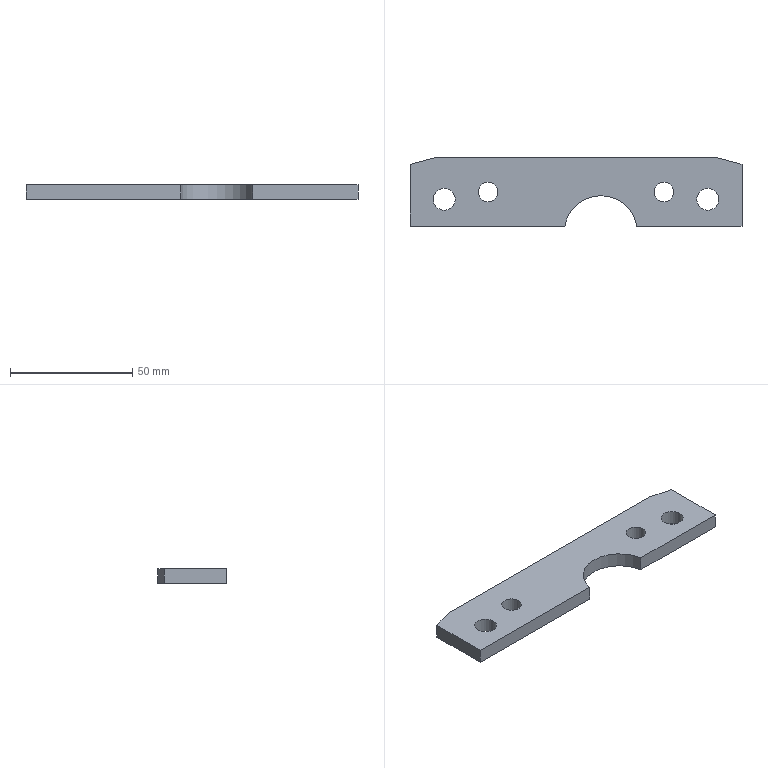Part | STEP file | gslz 2016.10.28-13_id714_x_t | 1 solid | 14 faces | box 136 x 28 x 6 mm | volume 19648 mm3 | plane 9 | cylinder 5 | commonest cylinder face diameters 8 x2 9 x2 30 x1
STEP:
#1=CARTESIAN_POINT('',(0.,0.,0.));
#2=DIRECTION('',(0.,0.,1.));
#3=DIRECTION('',(1.,0.,0.));
#4=AXIS2_PLACEMENT_3D('',#1,#2,#3);
#5=CARTESIAN_POINT('',(-122.555,-295.75,6.));
#6=VERTEX_POINT('',#5);
#7=CARTESIAN_POINT('',(-79.516,-295.75,6.));
#8=VERTEX_POINT('',#7);
#9=CARTESIAN_POINT('',(-142.516,-295.75,6.));
#10=DIRECTION('',(1.,0.,0.));
#11=VECTOR('',#10,1.);
#12=LINE('',#9,#11);
#13=CARTESIAN_POINT('',(-142.516,-295.75,16.));
#14=DIRECTION('',(0.,1.,0.));
#15=DIRECTION('',(0.,0.,-1.));
#16=AXIS2_PLACEMENT_3D('',#13,#14,#15);
#17=PLANE('',#16);
#18=CARTESIAN_POINT('',(10.,0.));
#19=DIRECTION('',(0.,-1.));
#20=VECTOR('',#19,1.);
#21=LINE('',#18,#20);
#22=(GEOMETRIC_REPRESENTATION_CONTEXT(2)PARAMETRIC_REPRESENTATION_CONTEXT()REPRESENTATION_CONTEXT('',''));
#23=DEFINITIONAL_REPRESENTATION('',(#21),#22);
#24=PCURVE('',#17,#23);
#25=CARTESIAN_POINT('',(-182.516,-265.25,6.));
#26=DIRECTION('',(0.,0.,-1.));
#27=DIRECTION('',(-1.,0.,0.));
#28=AXIS2_PLACEMENT_3D('',#25,#26,#27);
#29=PLANE('',#28);
#30=CARTESIAN_POINT('',(-40.,-30.5));
#31=DIRECTION('',(-1.,0.));
#32=VECTOR('',#31,1.);
#33=LINE('',#30,#32);
#34=(GEOMETRIC_REPRESENTATION_CONTEXT(2)PARAMETRIC_REPRESENTATION_CONTEXT()REPRESENTATION_CONTEXT('',''));
#35=DEFINITIONAL_REPRESENTATION('',(#33),#34);
#36=PCURVE('',#29,#35);
#37=SURFACE_CURVE('',#12,(#24,#36),.PCURVE_S1.);
#38=EDGE_CURVE('',#6,#8,#37,.T.);
#39=ORIENTED_EDGE('',*,*,#38,.F.);
#40=CARTESIAN_POINT('',(-122.555,-295.75,0.));
#41=VERTEX_POINT('',#40);
#42=CARTESIAN_POINT('',(-122.555,-295.75,290.));
#43=DIRECTION('',(0.,0.,-1.));
#44=VECTOR('',#43,1.);
#45=LINE('',#42,#44);
#46=CARTESIAN_POINT('',(-274.,-19.961));
#47=DIRECTION('',(1.,0.));
#48=VECTOR('',#47,1.);
#49=LINE('',#46,#48);
#50=(GEOMETRIC_REPRESENTATION_CONTEXT(2)PARAMETRIC_REPRESENTATION_CONTEXT()REPRESENTATION_CONTEXT('',''));
#51=DEFINITIONAL_REPRESENTATION('',(#49),#50);
#52=PCURVE('',#17,#51);
#53=CARTESIAN_POINT('',(-137.345,-298.25,290.));
#54=DIRECTION('',(0.,0.,-1.));
#55=DIRECTION('',(-1.,0.,0.));
#56=AXIS2_PLACEMENT_3D('',#53,#54,#55);
#57=CYLINDRICAL_SURFACE('',#56,15.);
#58=CARTESIAN_POINT('',(2.974,0.));
#59=DIRECTION('',(0.,1.));
#60=VECTOR('',#59,1.);
#61=LINE('',#58,#60);
#62=(GEOMETRIC_REPRESENTATION_CONTEXT(2)PARAMETRIC_REPRESENTATION_CONTEXT()REPRESENTATION_CONTEXT('',''));
#63=DEFINITIONAL_REPRESENTATION('',(#61),#62);
#64=PCURVE('',#57,#63);
#65=SURFACE_CURVE('',#45,(#52,#64),.PCURVE_S1.);
#66=EDGE_CURVE('',#6,#41,#65,.T.);
#67=ORIENTED_EDGE('',*,*,#66,.T.);
#68=CARTESIAN_POINT('',(-79.516,-295.75,0.));
#69=VERTEX_POINT('',#68);
#70=CARTESIAN_POINT('',(-142.516,-295.75,0.));
#71=DIRECTION('',(-1.,0.,0.));
#72=VECTOR('',#71,1.);
#73=LINE('',#70,#72);
#74=CARTESIAN_POINT('',(16.,0.));
#75=DIRECTION('',(0.,1.));
#76=VECTOR('',#75,1.);
#77=LINE('',#74,#76);
#78=(GEOMETRIC_REPRESENTATION_CONTEXT(2)PARAMETRIC_REPRESENTATION_CONTEXT()REPRESENTATION_CONTEXT('',''));
#79=DEFINITIONAL_REPRESENTATION('',(#77),#78);
#80=PCURVE('',#17,#79);
#81=CARTESIAN_POINT('',(-222.516,-295.75,0.));
#82=DIRECTION('',(0.,0.,1.));
#83=DIRECTION('',(1.,0.,0.));
#84=AXIS2_PLACEMENT_3D('',#81,#82,#83);
#85=PLANE('',#84);
#86=CARTESIAN_POINT('',(80.,0.));
#87=DIRECTION('',(-1.,0.));
#88=VECTOR('',#87,1.);
#89=LINE('',#86,#88);
#90=(GEOMETRIC_REPRESENTATION_CONTEXT(2)PARAMETRIC_REPRESENTATION_CONTEXT()REPRESENTATION_CONTEXT('',''));
#91=DEFINITIONAL_REPRESENTATION('',(#89),#90);
#92=PCURVE('',#85,#91);
#93=SURFACE_CURVE('',#73,(#80,#92),.PCURVE_S1.);
#94=EDGE_CURVE('',#69,#41,#93,.T.);
#95=ORIENTED_EDGE('',*,*,#94,.F.);
#96=CARTESIAN_POINT('',(-79.516,-295.75,16.));
#97=DIRECTION('',(0.,0.,-1.));
#98=VECTOR('',#97,1.);
#99=LINE('',#96,#98);
#100=CARTESIAN_POINT('',(0.,-63.));
#101=DIRECTION('',(1.,0.));
#102=VECTOR('',#101,1.);
#103=LINE('',#100,#102);
#104=(GEOMETRIC_REPRESENTATION_CONTEXT(2)PARAMETRIC_REPRESENTATION_CONTEXT()REPRESENTATION_CONTEXT('',''));
#105=DEFINITIONAL_REPRESENTATION('',(#103),#104);
#106=PCURVE('',#17,#105);
#107=CARTESIAN_POINT('',(-79.516,-262.75,16.));
#108=DIRECTION('',(-1.,0.,0.));
#109=DIRECTION('',(0.,0.,1.));
#110=AXIS2_PLACEMENT_3D('',#107,#108,#109);
#111=PLANE('',#110);
#112=CARTESIAN_POINT('',(0.,-33.));
#113=DIRECTION('',(-1.,0.));
#114=VECTOR('',#113,1.);
#115=LINE('',#112,#114);
#116=(GEOMETRIC_REPRESENTATION_CONTEXT(2)PARAMETRIC_REPRESENTATION_CONTEXT()REPRESENTATION_CONTEXT('',''));
#117=DEFINITIONAL_REPRESENTATION('',(#115),#116);
#118=PCURVE('',#111,#117);
#119=SURFACE_CURVE('',#99,(#106,#118),.PCURVE_S1.);
#120=EDGE_CURVE('',#8,#69,#119,.T.);
#121=ORIENTED_EDGE('',*,*,#120,.F.);
#122=EDGE_LOOP('',(#39,#67,#95,#121));
#123=FACE_BOUND('',#122,.T.);
#124=ADVANCED_FACE('',(#123),#17,.F.);
#125=CARTESIAN_POINT('',(-89.016,-284.75,0.));
#126=VERTEX_POINT('',#125);
#127=CARTESIAN_POINT('',(-98.016,-284.75,0.));
#128=VERTEX_POINT('',#127);
#129=CARTESIAN_POINT('',(-93.516,-284.75,0.));
#130=DIRECTION('',(0.,0.,1.));
#131=DIRECTION('',(1.,0.,0.));
#132=AXIS2_PLACEMENT_3D('',#129,#130,#131);
#133=CIRCLE('',#132,4.5);
#134=CARTESIAN_POINT('',(129.,11.));
#135=DIRECTION('',(1.,0.));
#136=AXIS2_PLACEMENT_2D('',#134,#135);
#137=CIRCLE('',#136,4.5);
#138=(GEOMETRIC_REPRESENTATION_CONTEXT(2)PARAMETRIC_REPRESENTATION_CONTEXT()REPRESENTATION_CONTEXT('',''));
#139=DEFINITIONAL_REPRESENTATION('',(#137),#138);
#140=PCURVE('',#85,#139);
#141=CARTESIAN_POINT('',(-93.516,-284.75,47.));
#142=DIRECTION('',(0.,0.,-1.));
#143=DIRECTION('',(-1.,0.,0.));
#144=AXIS2_PLACEMENT_3D('',#141,#142,#143);
#145=CYLINDRICAL_SURFACE('',#144,4.5);
#146=CARTESIAN_POINT('',(3.142,47.));
#147=DIRECTION('',(-1.,0.));
#148=VECTOR('',#147,1.);
#149=LINE('',#146,#148);
#150=(GEOMETRIC_REPRESENTATION_CONTEXT(2)PARAMETRIC_REPRESENTATION_CONTEXT()REPRESENTATION_CONTEXT('',''));
#151=DEFINITIONAL_REPRESENTATION('',(#149),#150);
#152=PCURVE('',#145,#151);
#153=SURFACE_CURVE('',#133,(#140,#152),.PCURVE_S1.);
#154=EDGE_CURVE('',#126,#128,#153,.T.);
#155=ORIENTED_EDGE('',*,*,#154,.T.);
#156=CARTESIAN_POINT('',(-93.516,-284.75,0.));
#157=DIRECTION('',(0.,0.,1.));
#158=DIRECTION('',(1.,0.,0.));
#159=AXIS2_PLACEMENT_3D('',#156,#157,#158);
#160=CIRCLE('',#159,4.5);
#161=CARTESIAN_POINT('',(129.,11.));
#162=DIRECTION('',(1.,0.));
#163=AXIS2_PLACEMENT_2D('',#161,#162);
#164=CIRCLE('',#163,4.5);
#165=(GEOMETRIC_REPRESENTATION_CONTEXT(2)PARAMETRIC_REPRESENTATION_CONTEXT()REPRESENTATION_CONTEXT('',''));
#166=DEFINITIONAL_REPRESENTATION('',(#164),#165);
#167=PCURVE('',#85,#166);
#168=CARTESIAN_POINT('',(9.425,47.));
#169=DIRECTION('',(-1.,0.));
#170=VECTOR('',#169,1.);
#171=LINE('',#168,#170);
#172=(GEOMETRIC_REPRESENTATION_CONTEXT(2)PARAMETRIC_REPRESENTATION_CONTEXT()REPRESENTATION_CONTEXT('',''));
#173=DEFINITIONAL_REPRESENTATION('',(#171),#172);
#174=PCURVE('',#145,#173);
#175=SURFACE_CURVE('',#160,(#167,#174),.PCURVE_S1.);
#176=EDGE_CURVE('',#128,#126,#175,.T.);
#177=ORIENTED_EDGE('',*,*,#176,.T.);
#178=EDGE_LOOP('',(#155,#177));
#179=FACE_BOUND('',#178,.T.);
#180=CARTESIAN_POINT('',(-179.516,-281.75,0.));
#181=VERTEX_POINT('',#180);
#182=CARTESIAN_POINT('',(-183.516,-281.75,0.));
#183=DIRECTION('',(0.,0.,1.));
#184=DIRECTION('',(1.,0.,0.));
#185=AXIS2_PLACEMENT_3D('',#182,#183,#184);
#186=CIRCLE('',#185,4.);
#187=CARTESIAN_POINT('',(39.,14.));
#188=DIRECTION('',(1.,0.));
#189=AXIS2_PLACEMENT_2D('',#187,#188);
#190=CIRCLE('',#189,4.);
#191=(GEOMETRIC_REPRESENTATION_CONTEXT(2)PARAMETRIC_REPRESENTATION_CONTEXT()REPRESENTATION_CONTEXT('',''));
#192=DEFINITIONAL_REPRESENTATION('',(#190),#191);
#193=PCURVE('',#85,#192);
#194=CARTESIAN_POINT('',(-183.516,-281.75,-73.));
#195=DIRECTION('',(0.,0.,1.));
#196=DIRECTION('',(1.,0.,0.));
#197=AXIS2_PLACEMENT_3D('',#194,#195,#196);
#198=CYLINDRICAL_SURFACE('',#197,4.);
#199=CARTESIAN_POINT('',(0.,73.));
#200=DIRECTION('',(1.,0.));
#201=VECTOR('',#200,1.);
#202=LINE('',#199,#201);
#203=(GEOMETRIC_REPRESENTATION_CONTEXT(2)PARAMETRIC_REPRESENTATION_CONTEXT()REPRESENTATION_CONTEXT('',''));
#204=DEFINITIONAL_REPRESENTATION('',(#202),#203);
#205=PCURVE('',#198,#204);
#206=SURFACE_CURVE('',#186,(#193,#205),.PCURVE_S1.);
#207=EDGE_CURVE('',#181,#181,#206,.T.);
#208=ORIENTED_EDGE('',*,*,#207,.T.);
#209=EDGE_LOOP('',(#208));
#210=FACE_BOUND('',#209,.T.);
#211=CARTESIAN_POINT('',(-107.516,-281.75,0.));
#212=VERTEX_POINT('',#211);
#213=CARTESIAN_POINT('',(-111.516,-281.75,0.));
#214=DIRECTION('',(0.,0.,-1.));
#215=DIRECTION('',(1.,0.,0.));
#216=AXIS2_PLACEMENT_3D('',#213,#214,#215);
#217=CIRCLE('',#216,4.);
#218=CARTESIAN_POINT('',(115.,14.));
#219=CARTESIAN_POINT('',(115.,7.072));
#220=CARTESIAN_POINT('',(109.,10.536));
#221=CARTESIAN_POINT('',(103.,14.));
#222=CARTESIAN_POINT('',(109.,17.464));
#223=CARTESIAN_POINT('',(115.,20.928));
#224=CARTESIAN_POINT('',(115.,14.));
#225=(BOUNDED_CURVE()B_SPLINE_CURVE(2,(#218,#219,#220,#221,#222,#223,#224),.UNSPECIFIED.,.T.,.F.)B_SPLINE_CURVE_WITH_KNOTS((1,2,2,2,2,1),(-2.094,0.,2.094,4.189,6.283,8.378),.UNSPECIFIED.)CURVE()GEOMETRIC_REPRESENTATION_ITEM()RATIONAL_B_SPLINE_CURVE((1.,0.5,1.,0.5,1.,0.5,1.))REPRESENTATION_ITEM(''));
#226=(GEOMETRIC_REPRESENTATION_CONTEXT(2)PARAMETRIC_REPRESENTATION_CONTEXT()REPRESENTATION_CONTEXT('',''));
#227=DEFINITIONAL_REPRESENTATION('',(#225),#226);
#228=PCURVE('',#85,#227);
#229=CARTESIAN_POINT('',(-111.516,-281.75,-73.));
#230=DIRECTION('',(0.,0.,1.));
#231=DIRECTION('',(1.,0.,0.));
#232=AXIS2_PLACEMENT_3D('',#229,#230,#231);
#233=CYLINDRICAL_SURFACE('',#232,4.);
#234=CARTESIAN_POINT('',(6.283,73.));
#235=DIRECTION('',(-1.,0.));
#236=VECTOR('',#235,1.);
#237=LINE('',#234,#236);
#238=(GEOMETRIC_REPRESENTATION_CONTEXT(2)PARAMETRIC_REPRESENTATION_CONTEXT()REPRESENTATION_CONTEXT('',''));
#239=DEFINITIONAL_REPRESENTATION('',(#237),#238);
#240=PCURVE('',#233,#239);
#241=SURFACE_CURVE('',#217,(#228,#240),.PCURVE_S1.);
#242=EDGE_CURVE('',#212,#212,#241,.T.);
#243=ORIENTED_EDGE('',*,*,#242,.F.);
#244=EDGE_LOOP('',(#243));
#245=FACE_BOUND('',#244,.T.);
#246=CARTESIAN_POINT('',(-197.016,-284.75,0.));
#247=VERTEX_POINT('',#246);
#248=CARTESIAN_POINT('',(-206.016,-284.75,0.));
#249=VERTEX_POINT('',#248);
#250=CARTESIAN_POINT('',(-201.516,-284.75,0.));
#251=DIRECTION('',(0.,0.,-1.));
#252=DIRECTION('',(1.,0.,0.));
#253=AXIS2_PLACEMENT_3D('',#250,#251,#252);
#254=CIRCLE('',#253,4.5);
#255=CARTESIAN_POINT('',(25.5,11.));
#256=CARTESIAN_POINT('',(25.5,3.206));
#257=CARTESIAN_POINT('',(18.75,7.103));
#258=CARTESIAN_POINT('',(12.,11.));
#259=CARTESIAN_POINT('',(18.75,14.897));
#260=CARTESIAN_POINT('',(25.5,18.794));
#261=CARTESIAN_POINT('',(25.5,11.));
#262=(BOUNDED_CURVE()B_SPLINE_CURVE(2,(#255,#256,#257,#258,#259,#260,#261),.UNSPECIFIED.,.T.,.F.)B_SPLINE_CURVE_WITH_KNOTS((1,2,2,2,2,1),(-2.094,0.,2.094,4.189,6.283,8.378),.UNSPECIFIED.)CURVE()GEOMETRIC_REPRESENTATION_ITEM()RATIONAL_B_SPLINE_CURVE((1.,0.5,1.,0.5,1.,0.5,1.))REPRESENTATION_ITEM(''));
#263=(GEOMETRIC_REPRESENTATION_CONTEXT(2)PARAMETRIC_REPRESENTATION_CONTEXT()REPRESENTATION_CONTEXT('',''));
#264=DEFINITIONAL_REPRESENTATION('',(#262),#263);
#265=PCURVE('',#85,#264);
#266=CARTESIAN_POINT('',(-201.516,-284.75,47.));
#267=DIRECTION('',(0.,0.,-1.));
#268=DIRECTION('',(-1.,0.,0.));
#269=AXIS2_PLACEMENT_3D('',#266,#267,#268);
#270=CYLINDRICAL_SURFACE('',#269,4.5);
#271=CARTESIAN_POINT('',(3.142,47.));
#272=DIRECTION('',(1.,0.));
#273=VECTOR('',#272,1.);
#274=LINE('',#271,#273);
#275=(GEOMETRIC_REPRESENTATION_CONTEXT(2)PARAMETRIC_REPRESENTATION_CONTEXT()REPRESENTATION_CONTEXT('',''));
#276=DEFINITIONAL_REPRESENTATION('',(#274),#275);
#277=PCURVE('',#270,#276);
#278=SURFACE_CURVE('',#254,(#265,#277),.PCURVE_S1.);
#279=EDGE_CURVE('',#247,#249,#278,.T.);
#280=ORIENTED_EDGE('',*,*,#279,.F.);
#281=CARTESIAN_POINT('',(-201.516,-284.75,0.));
#282=DIRECTION('',(0.,0.,-1.));
#283=DIRECTION('',(1.,0.,0.));
#284=AXIS2_PLACEMENT_3D('',#281,#282,#283);
#285=CIRCLE('',#284,4.5);
#286=CARTESIAN_POINT('',(25.5,11.));
#287=CARTESIAN_POINT('',(25.5,3.206));
#288=CARTESIAN_POINT('',(18.75,7.103));
#289=CARTESIAN_POINT('',(12.,11.));
#290=CARTESIAN_POINT('',(18.75,14.897));
#291=CARTESIAN_POINT('',(25.5,18.794));
#292=CARTESIAN_POINT('',(25.5,11.));
#293=(BOUNDED_CURVE()B_SPLINE_CURVE(2,(#286,#287,#288,#289,#290,#291,#292),.UNSPECIFIED.,.T.,.F.)B_SPLINE_CURVE_WITH_KNOTS((1,2,2,2,2,1),(-2.094,0.,2.094,4.189,6.283,8.378),.UNSPECIFIED.)CURVE()GEOMETRIC_REPRESENTATION_ITEM()RATIONAL_B_SPLINE_CURVE((1.,0.5,1.,0.5,1.,0.5,1.))REPRESENTATION_ITEM(''));
#294=(GEOMETRIC_REPRESENTATION_CONTEXT(2)PARAMETRIC_REPRESENTATION_CONTEXT()REPRESENTATION_CONTEXT('',''));
#295=DEFINITIONAL_REPRESENTATION('',(#293),#294);
#296=PCURVE('',#85,#295);
#297=CARTESIAN_POINT('',(-3.142,47.));
#298=DIRECTION('',(1.,0.));
#299=VECTOR('',#298,1.);
#300=LINE('',#297,#299);
#301=(GEOMETRIC_REPRESENTATION_CONTEXT(2)PARAMETRIC_REPRESENTATION_CONTEXT()REPRESENTATION_CONTEXT('',''));
#302=DEFINITIONAL_REPRESENTATION('',(#300),#301);
#303=PCURVE('',#270,#302);
#304=SURFACE_CURVE('',#285,(#296,#303),.PCURVE_S1.);
#305=EDGE_CURVE('',#249,#247,#304,.T.);
#306=ORIENTED_EDGE('',*,*,#305,.F.);
#307=EDGE_LOOP('',(#280,#306));
#308=FACE_BOUND('',#307,.T.);
#309=CARTESIAN_POINT('',(-152.135,-295.75,0.));
#310=VERTEX_POINT('',#309);
#311=CARTESIAN_POINT('',(-137.345,-298.25,0.));
#312=DIRECTION('',(0.,0.,-1.));
#313=DIRECTION('',(1.,0.,0.));
#314=AXIS2_PLACEMENT_3D('',#311,#312,#313);
#315=CIRCLE('',#314,15.);
#316=CARTESIAN_POINT('',(100.17,-2.5));
#317=CARTESIAN_POINT('',(100.17,-28.481));
#318=CARTESIAN_POINT('',(77.67,-15.49));
#319=CARTESIAN_POINT('',(55.17,-2.5));
#320=CARTESIAN_POINT('',(77.67,10.49));
#321=CARTESIAN_POINT('',(100.17,23.481));
#322=CARTESIAN_POINT('',(100.17,-2.5));
#323=(BOUNDED_CURVE()B_SPLINE_CURVE(2,(#316,#317,#318,#319,#320,#321,#322),.UNSPECIFIED.,.T.,.F.)B_SPLINE_CURVE_WITH_KNOTS((1,2,2,2,2,1),(-2.094,0.,2.094,4.189,6.283,8.378),.UNSPECIFIED.)CURVE()GEOMETRIC_REPRESENTATION_ITEM()RATIONAL_B_SPLINE_CURVE((1.,0.5,1.,0.5,1.,0.5,1.))REPRESENTATION_ITEM(''));
#324=(GEOMETRIC_REPRESENTATION_CONTEXT(2)PARAMETRIC_REPRESENTATION_CONTEXT()REPRESENTATION_CONTEXT('',''));
#325=DEFINITIONAL_REPRESENTATION('',(#323),#324);
#326=PCURVE('',#85,#325);
#327=CARTESIAN_POINT('',(-3.142,290.));
#328=DIRECTION('',(1.,0.));
#329=VECTOR('',#328,1.);
#330=LINE('',#327,#329);
#331=(GEOMETRIC_REPRESENTATION_CONTEXT(2)PARAMETRIC_REPRESENTATION_CONTEXT()REPRESENTATION_CONTEXT('',''));
#332=DEFINITIONAL_REPRESENTATION('',(#330),#331);
#333=PCURVE('',#57,#332);
#334=SURFACE_CURVE('',#315,(#326,#333),.PCURVE_S1.);
#335=EDGE_CURVE('',#310,#41,#334,.T.);
#336=ORIENTED_EDGE('',*,*,#335,.F.);
#337=CARTESIAN_POINT('',(-215.516,-295.75,0.));
#338=VERTEX_POINT('',#337);
#339=CARTESIAN_POINT('',(-142.516,-295.75,0.));
#340=DIRECTION('',(-1.,0.,0.));
#341=VECTOR('',#340,1.);
#342=LINE('',#339,#341);
#343=CARTESIAN_POINT('',(80.,0.));
#344=DIRECTION('',(-1.,0.));
#345=VECTOR('',#344,1.);
#346=LINE('',#343,#345);
#347=(GEOMETRIC_REPRESENTATION_CONTEXT(2)PARAMETRIC_REPRESENTATION_CONTEXT()REPRESENTATION_CONTEXT('',''));
#348=DEFINITIONAL_REPRESENTATION('',(#346),#347);
#349=PCURVE('',#85,#348);
#350=CARTESIAN_POINT('',(-142.516,-295.75,16.));
#351=DIRECTION('',(0.,1.,0.));
#352=DIRECTION('',(0.,0.,-1.));
#353=AXIS2_PLACEMENT_3D('',#350,#351,#352);
#354=PLANE('',#353);
#355=CARTESIAN_POINT('',(16.,0.));
#356=DIRECTION('',(0.,1.));
#357=VECTOR('',#356,1.);
#358=LINE('',#355,#357);
#359=(GEOMETRIC_REPRESENTATION_CONTEXT(2)PARAMETRIC_REPRESENTATION_CONTEXT()REPRESENTATION_CONTEXT('',''));
#360=DEFINITIONAL_REPRESENTATION('',(#358),#359);
#361=PCURVE('',#354,#360);
#362=SURFACE_CURVE('',#342,(#349,#361),.PCURVE_S1.);
#363=EDGE_CURVE('',#310,#338,#362,.T.);
#364=ORIENTED_EDGE('',*,*,#363,.T.);
#365=CARTESIAN_POINT('',(-215.516,-270.43,0.));
#366=VERTEX_POINT('',#365);
#367=CARTESIAN_POINT('',(-215.516,-295.75,0.));
#368=DIRECTION('',(0.,1.,0.));
#369=VECTOR('',#368,1.);
#370=LINE('',#367,#369);
#371=CARTESIAN_POINT('',(7.,0.));
#372=DIRECTION('',(0.,1.));
#373=VECTOR('',#372,1.);
#374=LINE('',#371,#373);
#375=(GEOMETRIC_REPRESENTATION_CONTEXT(2)PARAMETRIC_REPRESENTATION_CONTEXT()REPRESENTATION_CONTEXT('',''));
#376=DEFINITIONAL_REPRESENTATION('',(#374),#375);
#377=PCURVE('',#85,#376);
#378=CARTESIAN_POINT('',(-215.516,-295.75,16.));
#379=DIRECTION('',(1.,0.,0.));
#380=DIRECTION('',(0.,0.,-1.));
#381=AXIS2_PLACEMENT_3D('',#378,#379,#380);
#382=PLANE('',#381);
#383=CARTESIAN_POINT('',(16.,0.));
#384=DIRECTION('',(0.,1.));
#385=VECTOR('',#384,1.);
#386=LINE('',#383,#385);
#387=(GEOMETRIC_REPRESENTATION_CONTEXT(2)PARAMETRIC_REPRESENTATION_CONTEXT()REPRESENTATION_CONTEXT('',''));
#388=DEFINITIONAL_REPRESENTATION('',(#386),#387);
#389=PCURVE('',#382,#388);
#390=SURFACE_CURVE('',#370,(#377,#389),.PCURVE_S1.);
#391=EDGE_CURVE('',#338,#366,#390,.T.);
#392=ORIENTED_EDGE('',*,*,#391,.T.);
#393=CARTESIAN_POINT('',(-205.514,-267.75,0.));
#394=VERTEX_POINT('',#393);
#395=CARTESIAN_POINT('',(-215.516,-270.43,0.));
#396=DIRECTION('',(0.9659,0.2588,0.));
#397=VECTOR('',#396,1.);
#398=LINE('',#395,#397);
#399=CARTESIAN_POINT('',(7.,25.32));
#400=DIRECTION('',(0.9659,0.2588));
#401=VECTOR('',#400,1.);
#402=LINE('',#399,#401);
#403=(GEOMETRIC_REPRESENTATION_CONTEXT(2)PARAMETRIC_REPRESENTATION_CONTEXT()REPRESENTATION_CONTEXT('',''));
#404=DEFINITIONAL_REPRESENTATION('',(#402),#403);
#405=PCURVE('',#85,#404);
#406=CARTESIAN_POINT('',(-215.516,-270.43,8.));
#407=DIRECTION('',(0.2588,-0.9659,0.));
#408=DIRECTION('',(-0.9659,-0.2588,0.));
#409=AXIS2_PLACEMENT_3D('',#406,#407,#408);
#410=PLANE('',#409);
#411=CARTESIAN_POINT('',(0.,8.));
#412=DIRECTION('',(-1.,0.));
#413=VECTOR('',#412,1.);
#414=LINE('',#411,#413);
#415=(GEOMETRIC_REPRESENTATION_CONTEXT(2)PARAMETRIC_REPRESENTATION_CONTEXT()REPRESENTATION_CONTEXT('',''));
#416=DEFINITIONAL_REPRESENTATION('',(#414),#415);
#417=PCURVE('',#410,#416);
#418=SURFACE_CURVE('',#398,(#405,#417),.PCURVE_S1.);
#419=EDGE_CURVE('',#366,#394,#418,.T.);
#420=ORIENTED_EDGE('',*,*,#419,.T.);
#421=CARTESIAN_POINT('',(-89.515,-267.75,0.));
#422=VERTEX_POINT('',#421);
#423=CARTESIAN_POINT('',(-212.514,-267.75,0.));
#424=DIRECTION('',(1.,0.,0.));
#425=VECTOR('',#424,1.);
#426=LINE('',#423,#425);
#427=CARTESIAN_POINT('',(10.002,28.));
#428=DIRECTION('',(1.,0.));
#429=VECTOR('',#428,1.);
#430=LINE('',#427,#429);
#431=(GEOMETRIC_REPRESENTATION_CONTEXT(2)PARAMETRIC_REPRESENTATION_CONTEXT()REPRESENTATION_CONTEXT('',''));
#432=DEFINITIONAL_REPRESENTATION('',(#430),#431);
#433=PCURVE('',#85,#432);
#434=CARTESIAN_POINT('',(-212.514,-267.75,8.));
#435=DIRECTION('',(0.,-1.,0.));
#436=DIRECTION('',(0.,0.,1.));
#437=AXIS2_PLACEMENT_3D('',#434,#435,#436);
#438=PLANE('',#437);
#439=CARTESIAN_POINT('',(-8.,0.));
#440=DIRECTION('',(0.,-1.));
#441=VECTOR('',#440,1.);
#442=LINE('',#439,#441);
#443=(GEOMETRIC_REPRESENTATION_CONTEXT(2)PARAMETRIC_REPRESENTATION_CONTEXT()REPRESENTATION_CONTEXT('',''));
#444=DEFINITIONAL_REPRESENTATION('',(#442),#443);
#445=PCURVE('',#438,#444);
#446=SURFACE_CURVE('',#426,(#433,#445),.PCURVE_S1.);
#447=EDGE_CURVE('',#394,#422,#446,.T.);
#448=ORIENTED_EDGE('',*,*,#447,.T.);
#449=CARTESIAN_POINT('',(-79.516,-270.429,0.));
#450=VERTEX_POINT('',#449);
#451=CARTESIAN_POINT('',(-89.515,-267.75,0.));
#452=DIRECTION('',(0.9659,-0.2588,0.));
#453=VECTOR('',#452,1.);
#454=LINE('',#451,#453);
#455=CARTESIAN_POINT('',(133.001,28.));
#456=DIRECTION('',(0.9659,-0.2588));
#457=VECTOR('',#456,1.);
#458=LINE('',#455,#457);
#459=(GEOMETRIC_REPRESENTATION_CONTEXT(2)PARAMETRIC_REPRESENTATION_CONTEXT()REPRESENTATION_CONTEXT('',''));
#460=DEFINITIONAL_REPRESENTATION('',(#458),#459);
#461=PCURVE('',#85,#460);
#462=CARTESIAN_POINT('',(-89.515,-267.75,8.));
#463=DIRECTION('',(-0.2588,-0.9659,0.));
#464=DIRECTION('',(-0.9659,0.2588,0.));
#465=AXIS2_PLACEMENT_3D('',#462,#463,#464);
#466=PLANE('',#465);
#467=CARTESIAN_POINT('',(0.,8.));
#468=DIRECTION('',(-1.,0.));
#469=VECTOR('',#468,1.);
#470=LINE('',#467,#469);
#471=(GEOMETRIC_REPRESENTATION_CONTEXT(2)PARAMETRIC_REPRESENTATION_CONTEXT()REPRESENTATION_CONTEXT('',''));
#472=DEFINITIONAL_REPRESENTATION('',(#470),#471);
#473=PCURVE('',#466,#472);
#474=SURFACE_CURVE('',#454,(#461,#473),.PCURVE_S1.);
#475=EDGE_CURVE('',#422,#450,#474,.T.);
#476=ORIENTED_EDGE('',*,*,#475,.T.);
#477=CARTESIAN_POINT('',(-79.516,-262.75,0.));
#478=DIRECTION('',(0.,-1.,0.));
#479=VECTOR('',#478,1.);
#480=LINE('',#477,#479);
#481=CARTESIAN_POINT('',(143.,33.));
#482=DIRECTION('',(0.,-1.));
#483=VECTOR('',#482,1.);
#484=LINE('',#481,#483);
#485=(GEOMETRIC_REPRESENTATION_CONTEXT(2)PARAMETRIC_REPRESENTATION_CONTEXT()REPRESENTATION_CONTEXT('',''));
#486=DEFINITIONAL_REPRESENTATION('',(#484),#485);
#487=PCURVE('',#85,#486);
#488=CARTESIAN_POINT('',(-16.,0.));
#489=DIRECTION('',(0.,-1.));
#490=VECTOR('',#489,1.);
#491=LINE('',#488,#490);
#492=(GEOMETRIC_REPRESENTATION_CONTEXT(2)PARAMETRIC_REPRESENTATION_CONTEXT()REPRESENTATION_CONTEXT('',''));
#493=DEFINITIONAL_REPRESENTATION('',(#491),#492);
#494=PCURVE('',#111,#493);
#495=SURFACE_CURVE('',#480,(#487,#494),.PCURVE_S1.);
#496=EDGE_CURVE('',#450,#69,#495,.T.);
#497=ORIENTED_EDGE('',*,*,#496,.T.);
#498=ORIENTED_EDGE('',*,*,#94,.T.);
#499=EDGE_LOOP('',(#336,#364,#392,#420,#448,#476,#497,#498));
#500=FACE_BOUND('',#499,.T.);
#501=ADVANCED_FACE('',(#179,#210,#245,#308,#500),#85,.F.);
#502=CARTESIAN_POINT('',(-187.516,-281.75,6.));
#503=VERTEX_POINT('',#502);
#504=CARTESIAN_POINT('',(-179.516,-281.75,6.));
#505=VERTEX_POINT('',#504);
#506=CARTESIAN_POINT('',(-183.516,-281.75,6.));
#507=DIRECTION('',(0.,0.,-1.));
#508=DIRECTION('',(-1.,0.,0.));
#509=AXIS2_PLACEMENT_3D('',#506,#507,#508);
#510=CIRCLE('',#509,4.);
#511=CARTESIAN_POINT('',(3.142,79.));
#512=DIRECTION('',(-1.,0.));
#513=VECTOR('',#512,1.);
#514=LINE('',#511,#513);
#515=(GEOMETRIC_REPRESENTATION_CONTEXT(2)PARAMETRIC_REPRESENTATION_CONTEXT()REPRESENTATION_CONTEXT('',''));
#516=DEFINITIONAL_REPRESENTATION('',(#514),#515);
#517=PCURVE('',#198,#516);
#518=CARTESIAN_POINT('',(1.,-16.5));
#519=DIRECTION('',(1.,0.));
#520=AXIS2_PLACEMENT_2D('',#518,#519);
#521=CIRCLE('',#520,4.);
#522=(GEOMETRIC_REPRESENTATION_CONTEXT(2)PARAMETRIC_REPRESENTATION_CONTEXT()REPRESENTATION_CONTEXT('',''));
#523=DEFINITIONAL_REPRESENTATION('',(#521),#522);
#524=PCURVE('',#29,#523);
#525=SURFACE_CURVE('',#510,(#517,#524),.PCURVE_S1.);
#526=EDGE_CURVE('',#503,#505,#525,.T.);
#527=ORIENTED_EDGE('',*,*,#526,.T.);
#528=CARTESIAN_POINT('',(-179.516,-281.75,0.));
#529=CARTESIAN_POINT('',(-179.516,-281.75,6.));
#530=B_SPLINE_CURVE_WITH_KNOTS('',1,(#528,#529),.UNSPECIFIED.,.F.,.F.,(2,2),(73.,79.),.PIECEWISE_BEZIER_KNOTS.);
#531=CARTESIAN_POINT('',(0.,0.));
#532=DIRECTION('',(0.,1.));
#533=VECTOR('',#532,1.);
#534=LINE('',#531,#533);
#535=(GEOMETRIC_REPRESENTATION_CONTEXT(2)PARAMETRIC_REPRESENTATION_CONTEXT()REPRESENTATION_CONTEXT('',''));
#536=DEFINITIONAL_REPRESENTATION('',(#534),#535);
#537=PCURVE('',#198,#536);
#538=CARTESIAN_POINT('',(6.283,0.));
#539=DIRECTION('',(0.,1.));
#540=VECTOR('',#539,1.);
#541=LINE('',#538,#540);
#542=(GEOMETRIC_REPRESENTATION_CONTEXT(2)PARAMETRIC_REPRESENTATION_CONTEXT()REPRESENTATION_CONTEXT('',''));
#543=DEFINITIONAL_REPRESENTATION('',(#541),#542);
#544=PCURVE('',#198,#543);
#545=SEAM_CURVE('',#530,(#537,#544),.PCURVE_S1.);
#546=EDGE_CURVE('',#181,#505,#545,.T.);
#547=ORIENTED_EDGE('',*,*,#546,.F.);
#548=ORIENTED_EDGE('',*,*,#207,.T.);
#549=ORIENTED_EDGE('',*,*,#546,.T.);
#550=CARTESIAN_POINT('',(-183.516,-281.75,6.));
#551=DIRECTION('',(0.,0.,-1.));
#552=DIRECTION('',(-1.,0.,0.));
#553=AXIS2_PLACEMENT_3D('',#550,#551,#552);
#554=CIRCLE('',#553,4.);
#555=CARTESIAN_POINT('',(9.425,79.));
#556=DIRECTION('',(-1.,0.));
#557=VECTOR('',#556,1.);
#558=LINE('',#555,#557);
#559=(GEOMETRIC_REPRESENTATION_CONTEXT(2)PARAMETRIC_REPRESENTATION_CONTEXT()REPRESENTATION_CONTEXT('',''));
#560=DEFINITIONAL_REPRESENTATION('',(#558),#559);
#561=PCURVE('',#198,#560);
#562=CARTESIAN_POINT('',(1.,-16.5));
#563=DIRECTION('',(1.,0.));
#564=AXIS2_PLACEMENT_2D('',#562,#563);
#565=CIRCLE('',#564,4.);
#566=(GEOMETRIC_REPRESENTATION_CONTEXT(2)PARAMETRIC_REPRESENTATION_CONTEXT()REPRESENTATION_CONTEXT('',''));
#567=DEFINITIONAL_REPRESENTATION('',(#565),#566);
#568=PCURVE('',#29,#567);
#569=SURFACE_CURVE('',#554,(#561,#568),.PCURVE_S1.);
#570=EDGE_CURVE('',#505,#503,#569,.T.);
#571=ORIENTED_EDGE('',*,*,#570,.T.);
#572=EDGE_LOOP('',(#527,#547,#548,#549,#571));
#573=FACE_BOUND('',#572,.F.);
#574=ADVANCED_FACE('',(#573),#198,.F.);
#575=CARTESIAN_POINT('',(-107.516,-281.75,6.));
#576=VERTEX_POINT('',#575);
#577=CARTESIAN_POINT('',(-115.516,-281.75,6.));
#578=VERTEX_POINT('',#577);
#579=CARTESIAN_POINT('',(-111.516,-281.75,6.));
#580=DIRECTION('',(0.,0.,1.));
#581=DIRECTION('',(-1.,0.,0.));
#582=AXIS2_PLACEMENT_3D('',#579,#580,#581);
#583=CIRCLE('',#582,4.);
#584=CARTESIAN_POINT('',(-3.142,79.));
#585=DIRECTION('',(1.,0.));
#586=VECTOR('',#585,1.);
#587=LINE('',#584,#586);
#588=(GEOMETRIC_REPRESENTATION_CONTEXT(2)PARAMETRIC_REPRESENTATION_CONTEXT()REPRESENTATION_CONTEXT('',''));
#589=DEFINITIONAL_REPRESENTATION('',(#587),#588);
#590=PCURVE('',#233,#589);
#591=CARTESIAN_POINT('',(-67.,-16.5));
#592=CARTESIAN_POINT('',(-67.,-23.428));
#593=CARTESIAN_POINT('',(-73.,-19.964));
#594=CARTESIAN_POINT('',(-79.,-16.5));
#595=CARTESIAN_POINT('',(-73.,-13.036));
#596=CARTESIAN_POINT('',(-67.,-9.572));
#597=CARTESIAN_POINT('',(-67.,-16.5));
#598=(BOUNDED_CURVE()B_SPLINE_CURVE(2,(#591,#592,#593,#594,#595,#596,#597),.UNSPECIFIED.,.T.,.F.)B_SPLINE_CURVE_WITH_KNOTS((1,2,2,2,2,1),(-2.094,0.,2.094,4.189,6.283,8.378),.UNSPECIFIED.)CURVE()GEOMETRIC_REPRESENTATION_ITEM()RATIONAL_B_SPLINE_CURVE((1.,0.5,1.,0.5,1.,0.5,1.))REPRESENTATION_ITEM(''));
#599=(GEOMETRIC_REPRESENTATION_CONTEXT(2)PARAMETRIC_REPRESENTATION_CONTEXT()REPRESENTATION_CONTEXT('',''));
#600=DEFINITIONAL_REPRESENTATION('',(#598),#599);
#601=PCURVE('',#29,#600);
#602=SURFACE_CURVE('',#583,(#590,#601),.PCURVE_S1.);
#603=EDGE_CURVE('',#576,#578,#602,.T.);
#604=ORIENTED_EDGE('',*,*,#603,.F.);
#605=CARTESIAN_POINT('',(-107.516,-281.75,0.));
#606=CARTESIAN_POINT('',(-107.516,-281.75,6.));
#607=B_SPLINE_CURVE_WITH_KNOTS('',1,(#605,#606),.UNSPECIFIED.,.F.,.F.,(2,2),(73.,79.),.PIECEWISE_BEZIER_KNOTS.);
#608=CARTESIAN_POINT('',(0.,0.));
#609=DIRECTION('',(0.,1.));
#610=VECTOR('',#609,1.);
#611=LINE('',#608,#610);
#612=(GEOMETRIC_REPRESENTATION_CONTEXT(2)PARAMETRIC_REPRESENTATION_CONTEXT()REPRESENTATION_CONTEXT('',''));
#613=DEFINITIONAL_REPRESENTATION('',(#611),#612);
#614=PCURVE('',#233,#613);
#615=CARTESIAN_POINT('',(6.283,0.));
#616=DIRECTION('',(0.,1.));
#617=VECTOR('',#616,1.);
#618=LINE('',#615,#617);
#619=(GEOMETRIC_REPRESENTATION_CONTEXT(2)PARAMETRIC_REPRESENTATION_CONTEXT()REPRESENTATION_CONTEXT('',''));
#620=DEFINITIONAL_REPRESENTATION('',(#618),#619);
#621=PCURVE('',#233,#620);
#622=SEAM_CURVE('',#607,(#614,#621),.PCURVE_S1.);
#623=EDGE_CURVE('',#212,#576,#622,.T.);
#624=ORIENTED_EDGE('',*,*,#623,.F.);
#625=ORIENTED_EDGE('',*,*,#242,.F.);
#626=ORIENTED_EDGE('',*,*,#623,.T.);
#627=CARTESIAN_POINT('',(-111.516,-281.75,6.));
#628=DIRECTION('',(0.,0.,1.));
#629=DIRECTION('',(-1.,0.,0.));
#630=AXIS2_PLACEMENT_3D('',#627,#628,#629);
#631=CIRCLE('',#630,4.);
#632=CARTESIAN_POINT('',(3.142,79.));
#633=DIRECTION('',(1.,0.));
#634=VECTOR('',#633,1.);
#635=LINE('',#632,#634);
#636=(GEOMETRIC_REPRESENTATION_CONTEXT(2)PARAMETRIC_REPRESENTATION_CONTEXT()REPRESENTATION_CONTEXT('',''));
#637=DEFINITIONAL_REPRESENTATION('',(#635),#636);
#638=PCURVE('',#233,#637);
#639=CARTESIAN_POINT('',(-67.,-16.5));
#640=CARTESIAN_POINT('',(-67.,-23.428));
#641=CARTESIAN_POINT('',(-73.,-19.964));
#642=CARTESIAN_POINT('',(-79.,-16.5));
#643=CARTESIAN_POINT('',(-73.,-13.036));
#644=CARTESIAN_POINT('',(-67.,-9.572));
#645=CARTESIAN_POINT('',(-67.,-16.5));
#646=(BOUNDED_CURVE()B_SPLINE_CURVE(2,(#639,#640,#641,#642,#643,#644,#645),.UNSPECIFIED.,.T.,.F.)B_SPLINE_CURVE_WITH_KNOTS((1,2,2,2,2,1),(-2.094,0.,2.094,4.189,6.283,8.378),.UNSPECIFIED.)CURVE()GEOMETRIC_REPRESENTATION_ITEM()RATIONAL_B_SPLINE_CURVE((1.,0.5,1.,0.5,1.,0.5,1.))REPRESENTATION_ITEM(''));
#647=(GEOMETRIC_REPRESENTATION_CONTEXT(2)PARAMETRIC_REPRESENTATION_CONTEXT()REPRESENTATION_CONTEXT('',''));
#648=DEFINITIONAL_REPRESENTATION('',(#646),#647);
#649=PCURVE('',#29,#648);
#650=SURFACE_CURVE('',#631,(#638,#649),.PCURVE_S1.);
#651=EDGE_CURVE('',#578,#576,#650,.T.);
#652=ORIENTED_EDGE('',*,*,#651,.F.);
#653=EDGE_LOOP('',(#604,#624,#625,#626,#652));
#654=FACE_BOUND('',#653,.F.);
#655=ADVANCED_FACE('',(#654),#233,.F.);
#656=CARTESIAN_POINT('',(-206.016,-284.75,6.));
#657=VERTEX_POINT('',#656);
#658=CARTESIAN_POINT('',(-201.516,-284.75,6.));
#659=DIRECTION('',(0.,0.,1.));
#660=DIRECTION('',(-1.,0.,0.));
#661=AXIS2_PLACEMENT_3D('',#658,#659,#660);
#662=CIRCLE('',#661,4.5);
#663=CARTESIAN_POINT('',(6.283,41.));
#664=DIRECTION('',(-1.,0.));
#665=VECTOR('',#664,1.);
#666=LINE('',#663,#665);
#667=(GEOMETRIC_REPRESENTATION_CONTEXT(2)PARAMETRIC_REPRESENTATION_CONTEXT()REPRESENTATION_CONTEXT('',''));
#668=DEFINITIONAL_REPRESENTATION('',(#666),#667);
#669=PCURVE('',#270,#668);
#670=CARTESIAN_POINT('',(23.5,-19.5));
#671=CARTESIAN_POINT('',(23.5,-27.294));
#672=CARTESIAN_POINT('',(16.75,-23.397));
#673=CARTESIAN_POINT('',(10.,-19.5));
#674=CARTESIAN_POINT('',(16.75,-15.603));
#675=CARTESIAN_POINT('',(23.5,-11.706));
#676=CARTESIAN_POINT('',(23.5,-19.5));
#677=(BOUNDED_CURVE()B_SPLINE_CURVE(2,(#670,#671,#672,#673,#674,#675,#676),.UNSPECIFIED.,.T.,.F.)B_SPLINE_CURVE_WITH_KNOTS((1,2,2,2,2,1),(-2.094,0.,2.094,4.189,6.283,8.378),.UNSPECIFIED.)CURVE()GEOMETRIC_REPRESENTATION_ITEM()RATIONAL_B_SPLINE_CURVE((1.,0.5,1.,0.5,1.,0.5,1.))REPRESENTATION_ITEM(''));
#678=(GEOMETRIC_REPRESENTATION_CONTEXT(2)PARAMETRIC_REPRESENTATION_CONTEXT()REPRESENTATION_CONTEXT('',''));
#679=DEFINITIONAL_REPRESENTATION('',(#677),#678);
#680=PCURVE('',#29,#679);
#681=SURFACE_CURVE('',#662,(#669,#680),.PCURVE_S1.);
#682=EDGE_CURVE('',#657,#657,#681,.T.);
#683=ORIENTED_EDGE('',*,*,#682,.F.);
#684=CARTESIAN_POINT('',(-206.016,-284.75,6.));
#685=CARTESIAN_POINT('',(-206.016,-284.75,0.));
#686=B_SPLINE_CURVE_WITH_KNOTS('',1,(#684,#685),.UNSPECIFIED.,.F.,.F.,(2,2),(41.,47.),.PIECEWISE_BEZIER_KNOTS.);
#687=CARTESIAN_POINT('',(6.283,0.));
#688=DIRECTION('',(0.,1.));
#689=VECTOR('',#688,1.);
#690=LINE('',#687,#689);
#691=(GEOMETRIC_REPRESENTATION_CONTEXT(2)PARAMETRIC_REPRESENTATION_CONTEXT()REPRESENTATION_CONTEXT('',''));
#692=DEFINITIONAL_REPRESENTATION('',(#690),#691);
#693=PCURVE('',#270,#692);
#694=CARTESIAN_POINT('',(0.,0.));
#695=DIRECTION('',(0.,1.));
#696=VECTOR('',#695,1.);
#697=LINE('',#694,#696);
#698=(GEOMETRIC_REPRESENTATION_CONTEXT(2)PARAMETRIC_REPRESENTATION_CONTEXT()REPRESENTATION_CONTEXT('',''));
#699=DEFINITIONAL_REPRESENTATION('',(#697),#698);
#700=PCURVE('',#270,#699);
#701=SEAM_CURVE('',#686,(#693,#700),.PCURVE_S1.);
#702=EDGE_CURVE('',#657,#249,#701,.T.);
#703=ORIENTED_EDGE('',*,*,#702,.T.);
#704=ORIENTED_EDGE('',*,*,#279,.F.);
#705=ORIENTED_EDGE('',*,*,#305,.F.);
#706=ORIENTED_EDGE('',*,*,#702,.F.);
#707=EDGE_LOOP('',(#683,#703,#704,#705,#706));
#708=FACE_BOUND('',#707,.F.);
#709=ADVANCED_FACE('',(#708),#270,.F.);
#710=CARTESIAN_POINT('',(-89.515,-267.75,6.));
#711=VERTEX_POINT('',#710);
#712=CARTESIAN_POINT('',(-89.515,-267.75,8.));
#713=DIRECTION('',(0.,0.,1.));
#714=VECTOR('',#713,1.);
#715=LINE('',#712,#714);
#716=CARTESIAN_POINT('',(0.,-122.999));
#717=DIRECTION('',(1.,0.));
#718=VECTOR('',#717,1.);
#719=LINE('',#716,#718);
#720=(GEOMETRIC_REPRESENTATION_CONTEXT(2)PARAMETRIC_REPRESENTATION_CONTEXT()REPRESENTATION_CONTEXT('',''));
#721=DEFINITIONAL_REPRESENTATION('',(#719),#720);
#722=PCURVE('',#438,#721);
#723=CARTESIAN_POINT('',(0.,0.));
#724=DIRECTION('',(0.,-1.));
#725=VECTOR('',#724,1.);
#726=LINE('',#723,#725);
#727=(GEOMETRIC_REPRESENTATION_CONTEXT(2)PARAMETRIC_REPRESENTATION_CONTEXT()REPRESENTATION_CONTEXT('',''));
#728=DEFINITIONAL_REPRESENTATION('',(#726),#727);
#729=PCURVE('',#466,#728);
#730=SURFACE_CURVE('',#715,(#722,#729),.PCURVE_S1.);
#731=EDGE_CURVE('',#422,#711,#730,.T.);
#732=ORIENTED_EDGE('',*,*,#731,.F.);
#733=ORIENTED_EDGE('',*,*,#447,.F.);
#734=CARTESIAN_POINT('',(-205.514,-267.75,6.));
#735=VERTEX_POINT('',#734);
#736=CARTESIAN_POINT('',(-205.514,-267.75,8.));
#737=DIRECTION('',(0.,0.,1.));
#738=VECTOR('',#737,1.);
#739=LINE('',#736,#738);
#740=CARTESIAN_POINT('',(0.,-7.));
#741=DIRECTION('',(1.,0.));
#742=VECTOR('',#741,1.);
#743=LINE('',#740,#742);
#744=(GEOMETRIC_REPRESENTATION_CONTEXT(2)PARAMETRIC_REPRESENTATION_CONTEXT()REPRESENTATION_CONTEXT('',''));
#745=DEFINITIONAL_REPRESENTATION('',(#743),#744);
#746=PCURVE('',#438,#745);
#747=CARTESIAN_POINT('',(-10.355,0.));
#748=DIRECTION('',(0.,-1.));
#749=VECTOR('',#748,1.);
#750=LINE('',#747,#749);
#751=(GEOMETRIC_REPRESENTATION_CONTEXT(2)PARAMETRIC_REPRESENTATION_CONTEXT()REPRESENTATION_CONTEXT('',''));
#752=DEFINITIONAL_REPRESENTATION('',(#750),#751);
#753=PCURVE('',#410,#752);
#754=SURFACE_CURVE('',#739,(#746,#753),.PCURVE_S1.);
#755=EDGE_CURVE('',#394,#735,#754,.T.);
#756=ORIENTED_EDGE('',*,*,#755,.T.);
#757=CARTESIAN_POINT('',(-212.514,-267.75,6.));
#758=DIRECTION('',(-1.,0.,0.));
#759=VECTOR('',#758,1.);
#760=LINE('',#757,#759);
#761=CARTESIAN_POINT('',(-2.,0.));
#762=DIRECTION('',(0.,1.));
#763=VECTOR('',#762,1.);
#764=LINE('',#761,#763);
#765=(GEOMETRIC_REPRESENTATION_CONTEXT(2)PARAMETRIC_REPRESENTATION_CONTEXT()REPRESENTATION_CONTEXT('',''));
#766=DEFINITIONAL_REPRESENTATION('',(#764),#765);
#767=PCURVE('',#438,#766);
#768=CARTESIAN_POINT('',(29.998,-2.5));
#769=DIRECTION('',(1.,0.));
#770=VECTOR('',#769,1.);
#771=LINE('',#768,#770);
#772=(GEOMETRIC_REPRESENTATION_CONTEXT(2)PARAMETRIC_REPRESENTATION_CONTEXT()REPRESENTATION_CONTEXT('',''));
#773=DEFINITIONAL_REPRESENTATION('',(#771),#772);
#774=PCURVE('',#29,#773);
#775=SURFACE_CURVE('',#760,(#767,#774),.PCURVE_S1.);
#776=EDGE_CURVE('',#711,#735,#775,.T.);
#777=ORIENTED_EDGE('',*,*,#776,.F.);
#778=EDGE_LOOP('',(#732,#733,#756,#777));
#779=FACE_BOUND('',#778,.T.);
#780=ADVANCED_FACE('',(#779),#438,.F.);
#781=CARTESIAN_POINT('',(-79.516,-270.429,6.));
#782=VERTEX_POINT('',#781);
#783=CARTESIAN_POINT('',(-79.516,-270.429,8.));
#784=DIRECTION('',(0.,0.,-1.));
#785=VECTOR('',#784,1.);
#786=LINE('',#783,#785);
#787=CARTESIAN_POINT('',(-10.352,0.));
#788=DIRECTION('',(0.,1.));
#789=VECTOR('',#788,1.);
#790=LINE('',#787,#789);
#791=(GEOMETRIC_REPRESENTATION_CONTEXT(2)PARAMETRIC_REPRESENTATION_CONTEXT()REPRESENTATION_CONTEXT('',''));
#792=DEFINITIONAL_REPRESENTATION('',(#790),#791);
#793=PCURVE('',#466,#792);
#794=CARTESIAN_POINT('',(-8.,-7.679));
#795=DIRECTION('',(-1.,0.));
#796=VECTOR('',#795,1.);
#797=LINE('',#794,#796);
#798=(GEOMETRIC_REPRESENTATION_CONTEXT(2)PARAMETRIC_REPRESENTATION_CONTEXT()REPRESENTATION_CONTEXT('',''));
#799=DEFINITIONAL_REPRESENTATION('',(#797),#798);
#800=PCURVE('',#111,#799);
#801=SURFACE_CURVE('',#786,(#793,#800),.PCURVE_S1.);
#802=EDGE_CURVE('',#782,#450,#801,.T.);
#803=ORIENTED_EDGE('',*,*,#802,.T.);
#804=ORIENTED_EDGE('',*,*,#475,.F.);
#805=ORIENTED_EDGE('',*,*,#731,.T.);
#806=CARTESIAN_POINT('',(-89.515,-267.75,6.));
#807=DIRECTION('',(-0.9659,0.2588,0.));
#808=VECTOR('',#807,1.);
#809=LINE('',#806,#808);
#810=CARTESIAN_POINT('',(0.,2.));
#811=DIRECTION('',(1.,0.));
#812=VECTOR('',#811,1.);
#813=LINE('',#810,#812);
#814=(GEOMETRIC_REPRESENTATION_CONTEXT(2)PARAMETRIC_REPRESENTATION_CONTEXT()REPRESENTATION_CONTEXT('',''));
#815=DEFINITIONAL_REPRESENTATION('',(#813),#814);
#816=PCURVE('',#466,#815);
#817=CARTESIAN_POINT('',(-93.001,-2.5));
#818=DIRECTION('',(0.9659,0.2588));
#819=VECTOR('',#818,1.);
#820=LINE('',#817,#819);
#821=(GEOMETRIC_REPRESENTATION_CONTEXT(2)PARAMETRIC_REPRESENTATION_CONTEXT()REPRESENTATION_CONTEXT('',''));
#822=DEFINITIONAL_REPRESENTATION('',(#820),#821);
#823=PCURVE('',#29,#822);
#824=SURFACE_CURVE('',#809,(#816,#823),.PCURVE_S1.);
#825=EDGE_CURVE('',#782,#711,#824,.T.);
#826=ORIENTED_EDGE('',*,*,#825,.F.);
#827=EDGE_LOOP('',(#803,#804,#805,#826));
#828=FACE_BOUND('',#827,.T.);
#829=ADVANCED_FACE('',(#828),#466,.F.);
#830=ORIENTED_EDGE('',*,*,#120,.T.);
#831=ORIENTED_EDGE('',*,*,#496,.F.);
#832=ORIENTED_EDGE('',*,*,#802,.F.);
#833=CARTESIAN_POINT('',(-79.516,-262.75,6.));
#834=DIRECTION('',(0.,1.,0.));
#835=VECTOR('',#834,1.);
#836=LINE('',#833,#835);
#837=CARTESIAN_POINT('',(-10.,0.));
#838=DIRECTION('',(0.,1.));
#839=VECTOR('',#838,1.);
#840=LINE('',#837,#839);
#841=(GEOMETRIC_REPRESENTATION_CONTEXT(2)PARAMETRIC_REPRESENTATION_CONTEXT()REPRESENTATION_CONTEXT('',''));
#842=DEFINITIONAL_REPRESENTATION('',(#840),#841);
#843=PCURVE('',#111,#842);
#844=CARTESIAN_POINT('',(-103.,2.5));
#845=DIRECTION('',(0.,1.));
#846=VECTOR('',#845,1.);
#847=LINE('',#844,#846);
#848=(GEOMETRIC_REPRESENTATION_CONTEXT(2)PARAMETRIC_REPRESENTATION_CONTEXT()REPRESENTATION_CONTEXT('',''));
#849=DEFINITIONAL_REPRESENTATION('',(#847),#848);
#850=PCURVE('',#29,#849);
#851=SURFACE_CURVE('',#836,(#843,#850),.PCURVE_S1.);
#852=EDGE_CURVE('',#8,#782,#851,.T.);
#853=ORIENTED_EDGE('',*,*,#852,.F.);
#854=EDGE_LOOP('',(#830,#831,#832,#853));
#855=FACE_BOUND('',#854,.T.);
#856=ADVANCED_FACE('',(#855),#111,.F.);
#857=ORIENTED_EDGE('',*,*,#363,.F.);
#858=CARTESIAN_POINT('',(-152.135,-295.75,6.));
#859=VERTEX_POINT('',#858);
#860=CARTESIAN_POINT('',(-152.135,-295.75,290.));
#861=DIRECTION('',(0.,0.,1.));
#862=VECTOR('',#861,1.);
#863=LINE('',#860,#862);
#864=CARTESIAN_POINT('',(-274.,9.62));
#865=DIRECTION('',(-1.,0.));
#866=VECTOR('',#865,1.);
#867=LINE('',#864,#866);
#868=(GEOMETRIC_REPRESENTATION_CONTEXT(2)PARAMETRIC_REPRESENTATION_CONTEXT()REPRESENTATION_CONTEXT('',''));
#869=DEFINITIONAL_REPRESENTATION('',(#867),#868);
#870=PCURVE('',#354,#869);
#871=CARTESIAN_POINT('',(0.1674,0.));
#872=DIRECTION('',(0.,-1.));
#873=VECTOR('',#872,1.);
#874=LINE('',#871,#873);
#875=(GEOMETRIC_REPRESENTATION_CONTEXT(2)PARAMETRIC_REPRESENTATION_CONTEXT()REPRESENTATION_CONTEXT('',''));
#876=DEFINITIONAL_REPRESENTATION('',(#874),#875);
#877=PCURVE('',#57,#876);
#878=SURFACE_CURVE('',#863,(#870,#877),.PCURVE_S1.);
#879=EDGE_CURVE('',#310,#859,#878,.T.);
#880=ORIENTED_EDGE('',*,*,#879,.T.);
#881=CARTESIAN_POINT('',(-215.516,-295.75,6.));
#882=VERTEX_POINT('',#881);
#883=CARTESIAN_POINT('',(-142.516,-295.75,6.));
#884=DIRECTION('',(1.,0.,0.));
#885=VECTOR('',#884,1.);
#886=LINE('',#883,#885);
#887=CARTESIAN_POINT('',(10.,0.));
#888=DIRECTION('',(0.,-1.));
#889=VECTOR('',#888,1.);
#890=LINE('',#887,#889);
#891=(GEOMETRIC_REPRESENTATION_CONTEXT(2)PARAMETRIC_REPRESENTATION_CONTEXT()REPRESENTATION_CONTEXT('',''));
#892=DEFINITIONAL_REPRESENTATION('',(#890),#891);
#893=PCURVE('',#354,#892);
#894=CARTESIAN_POINT('',(-40.,-30.5));
#895=DIRECTION('',(-1.,0.));
#896=VECTOR('',#895,1.);
#897=LINE('',#894,#896);
#898=(GEOMETRIC_REPRESENTATION_CONTEXT(2)PARAMETRIC_REPRESENTATION_CONTEXT()REPRESENTATION_CONTEXT('',''));
#899=DEFINITIONAL_REPRESENTATION('',(#897),#898);
#900=PCURVE('',#29,#899);
#901=SURFACE_CURVE('',#886,(#893,#900),.PCURVE_S1.);
#902=EDGE_CURVE('',#882,#859,#901,.T.);
#903=ORIENTED_EDGE('',*,*,#902,.F.);
#904=CARTESIAN_POINT('',(-215.516,-295.75,16.));
#905=DIRECTION('',(0.,0.,-1.));
#906=VECTOR('',#905,1.);
#907=LINE('',#904,#906);
#908=CARTESIAN_POINT('',(0.,73.));
#909=DIRECTION('',(1.,0.));
#910=VECTOR('',#909,1.);
#911=LINE('',#908,#910);
#912=(GEOMETRIC_REPRESENTATION_CONTEXT(2)PARAMETRIC_REPRESENTATION_CONTEXT()REPRESENTATION_CONTEXT('',''));
#913=DEFINITIONAL_REPRESENTATION('',(#911),#912);
#914=PCURVE('',#354,#913);
#915=CARTESIAN_POINT('',(0.,0.));
#916=DIRECTION('',(1.,0.));
#917=VECTOR('',#916,1.);
#918=LINE('',#915,#917);
#919=(GEOMETRIC_REPRESENTATION_CONTEXT(2)PARAMETRIC_REPRESENTATION_CONTEXT()REPRESENTATION_CONTEXT('',''));
#920=DEFINITIONAL_REPRESENTATION('',(#918),#919);
#921=PCURVE('',#382,#920);
#922=SURFACE_CURVE('',#907,(#914,#921),.PCURVE_S1.);
#923=EDGE_CURVE('',#882,#338,#922,.T.);
#924=ORIENTED_EDGE('',*,*,#923,.T.);
#925=EDGE_LOOP('',(#857,#880,#903,#924));
#926=FACE_BOUND('',#925,.T.);
#927=ADVANCED_FACE('',(#926),#354,.F.);
#928=CARTESIAN_POINT('',(-215.516,-270.43,6.));
#929=VERTEX_POINT('',#928);
#930=CARTESIAN_POINT('',(-215.516,-270.43,8.));
#931=DIRECTION('',(0.,0.,-1.));
#932=VECTOR('',#931,1.);
#933=LINE('',#930,#932);
#934=CARTESIAN_POINT('',(8.,25.32));
#935=DIRECTION('',(1.,0.));
#936=VECTOR('',#935,1.);
#937=LINE('',#934,#936);
#938=(GEOMETRIC_REPRESENTATION_CONTEXT(2)PARAMETRIC_REPRESENTATION_CONTEXT()REPRESENTATION_CONTEXT('',''));
#939=DEFINITIONAL_REPRESENTATION('',(#937),#938);
#940=PCURVE('',#382,#939);
#941=CARTESIAN_POINT('',(0.,0.));
#942=DIRECTION('',(0.,1.));
#943=VECTOR('',#942,1.);
#944=LINE('',#941,#943);
#945=(GEOMETRIC_REPRESENTATION_CONTEXT(2)PARAMETRIC_REPRESENTATION_CONTEXT()REPRESENTATION_CONTEXT('',''));
#946=DEFINITIONAL_REPRESENTATION('',(#944),#945);
#947=PCURVE('',#410,#946);
#948=SURFACE_CURVE('',#933,(#940,#947),.PCURVE_S1.);
#949=EDGE_CURVE('',#929,#366,#948,.T.);
#950=ORIENTED_EDGE('',*,*,#949,.T.);
#951=ORIENTED_EDGE('',*,*,#391,.F.);
#952=ORIENTED_EDGE('',*,*,#923,.F.);
#953=CARTESIAN_POINT('',(-215.516,-295.75,6.));
#954=DIRECTION('',(0.,-1.,0.));
#955=VECTOR('',#954,1.);
#956=LINE('',#953,#955);
#957=CARTESIAN_POINT('',(10.,0.));
#958=DIRECTION('',(0.,-1.));
#959=VECTOR('',#958,1.);
#960=LINE('',#957,#959);
#961=(GEOMETRIC_REPRESENTATION_CONTEXT(2)PARAMETRIC_REPRESENTATION_CONTEXT()REPRESENTATION_CONTEXT('',''));
#962=DEFINITIONAL_REPRESENTATION('',(#960),#961);
#963=PCURVE('',#382,#962);
#964=CARTESIAN_POINT('',(33.,-30.5));
#965=DIRECTION('',(0.,-1.));
#966=VECTOR('',#965,1.);
#967=LINE('',#964,#966);
#968=(GEOMETRIC_REPRESENTATION_CONTEXT(2)PARAMETRIC_REPRESENTATION_CONTEXT()REPRESENTATION_CONTEXT('',''));
#969=DEFINITIONAL_REPRESENTATION('',(#967),#968);
#970=PCURVE('',#29,#969);
#971=SURFACE_CURVE('',#956,(#963,#970),.PCURVE_S1.);
#972=EDGE_CURVE('',#929,#882,#971,.T.);
#973=ORIENTED_EDGE('',*,*,#972,.F.);
#974=EDGE_LOOP('',(#950,#951,#952,#973));
#975=FACE_BOUND('',#974,.T.);
#976=ADVANCED_FACE('',(#975),#382,.F.);
#977=ORIENTED_EDGE('',*,*,#755,.F.);
#978=ORIENTED_EDGE('',*,*,#419,.F.);
#979=ORIENTED_EDGE('',*,*,#949,.F.);
#980=CARTESIAN_POINT('',(-215.516,-270.43,6.));
#981=DIRECTION('',(-0.9659,-0.2588,0.));
#982=VECTOR('',#981,1.);
#983=LINE('',#980,#982);
#984=CARTESIAN_POINT('',(0.,2.));
#985=DIRECTION('',(1.,0.));
#986=VECTOR('',#985,1.);
#987=LINE('',#984,#986);
#988=(GEOMETRIC_REPRESENTATION_CONTEXT(2)PARAMETRIC_REPRESENTATION_CONTEXT()REPRESENTATION_CONTEXT('',''));
#989=DEFINITIONAL_REPRESENTATION('',(#987),#988);
#990=PCURVE('',#410,#989);
#991=CARTESIAN_POINT('',(33.,-5.18));
#992=DIRECTION('',(0.9659,-0.2588));
#993=VECTOR('',#992,1.);
#994=LINE('',#991,#993);
#995=(GEOMETRIC_REPRESENTATION_CONTEXT(2)PARAMETRIC_REPRESENTATION_CONTEXT()REPRESENTATION_CONTEXT('',''));
#996=DEFINITIONAL_REPRESENTATION('',(#994),#995);
#997=PCURVE('',#29,#996);
#998=SURFACE_CURVE('',#983,(#990,#997),.PCURVE_S1.);
#999=EDGE_CURVE('',#735,#929,#998,.T.);
#1000=ORIENTED_EDGE('',*,*,#999,.F.);
#1001=EDGE_LOOP('',(#977,#978,#979,#1000));
#1002=FACE_BOUND('',#1001,.T.);
#1003=ADVANCED_FACE('',(#1002),#410,.F.);
#1004=ORIENTED_EDGE('',*,*,#902,.T.);
#1005=CARTESIAN_POINT('',(-137.345,-298.25,6.));
#1006=DIRECTION('',(0.,0.,-1.));
#1007=DIRECTION('',(-1.,0.,0.));
#1008=AXIS2_PLACEMENT_3D('',#1005,#1006,#1007);
#1009=CIRCLE('',#1008,15.);
#1010=CARTESIAN_POINT('',(-45.17,-33.));
#1011=DIRECTION('',(1.,0.));
#1012=AXIS2_PLACEMENT_2D('',#1010,#1011);
#1013=CIRCLE('',#1012,15.);
#1014=(GEOMETRIC_REPRESENTATION_CONTEXT(2)PARAMETRIC_REPRESENTATION_CONTEXT()REPRESENTATION_CONTEXT('',''));
#1015=DEFINITIONAL_REPRESENTATION('',(#1013),#1014);
#1016=PCURVE('',#29,#1015);
#1017=CARTESIAN_POINT('',(0.,284.));
#1018=DIRECTION('',(1.,0.));
#1019=VECTOR('',#1018,1.);
#1020=LINE('',#1017,#1019);
#1021=(GEOMETRIC_REPRESENTATION_CONTEXT(2)PARAMETRIC_REPRESENTATION_CONTEXT()REPRESENTATION_CONTEXT('',''));
#1022=DEFINITIONAL_REPRESENTATION('',(#1020),#1021);
#1023=PCURVE('',#57,#1022);
#1024=SURFACE_CURVE('',#1009,(#1016,#1023),.PCURVE_S1.);
#1025=EDGE_CURVE('',#859,#6,#1024,.T.);
#1026=ORIENTED_EDGE('',*,*,#1025,.T.);
#1027=ORIENTED_EDGE('',*,*,#38,.T.);
#1028=ORIENTED_EDGE('',*,*,#852,.T.);
#1029=ORIENTED_EDGE('',*,*,#825,.T.);
#1030=ORIENTED_EDGE('',*,*,#776,.T.);
#1031=ORIENTED_EDGE('',*,*,#999,.T.);
#1032=ORIENTED_EDGE('',*,*,#972,.T.);
#1033=EDGE_LOOP('',(#1004,#1026,#1027,#1028,#1029,#1030,#1031,#1032));
#1034=FACE_BOUND('',#1033,.T.);
#1035=ORIENTED_EDGE('',*,*,#682,.F.);
#1036=EDGE_LOOP('',(#1035));
#1037=FACE_BOUND('',#1036,.T.);
#1038=ORIENTED_EDGE('',*,*,#651,.F.);
#1039=ORIENTED_EDGE('',*,*,#603,.F.);
#1040=EDGE_LOOP('',(#1038,#1039));
#1041=FACE_BOUND('',#1040,.T.);
#1042=ORIENTED_EDGE('',*,*,#526,.T.);
#1043=ORIENTED_EDGE('',*,*,#570,.T.);
#1044=EDGE_LOOP('',(#1042,#1043));
#1045=FACE_BOUND('',#1044,.T.);
#1046=CARTESIAN_POINT('',(-98.016,-284.75,6.));
#1047=VERTEX_POINT('',#1046);
#1048=CARTESIAN_POINT('',(-93.516,-284.75,6.));
#1049=DIRECTION('',(0.,0.,-1.));
#1050=DIRECTION('',(-1.,0.,0.));
#1051=AXIS2_PLACEMENT_3D('',#1048,#1049,#1050);
#1052=CIRCLE('',#1051,4.5);
#1053=CARTESIAN_POINT('',(-89.,-19.5));
#1054=DIRECTION('',(1.,0.));
#1055=AXIS2_PLACEMENT_2D('',#1053,#1054);
#1056=CIRCLE('',#1055,4.5);
#1057=(GEOMETRIC_REPRESENTATION_CONTEXT(2)PARAMETRIC_REPRESENTATION_CONTEXT()REPRESENTATION_CONTEXT('',''));
#1058=DEFINITIONAL_REPRESENTATION('',(#1056),#1057);
#1059=PCURVE('',#29,#1058);
#1060=CARTESIAN_POINT('',(0.,41.));
#1061=DIRECTION('',(1.,0.));
#1062=VECTOR('',#1061,1.);
#1063=LINE('',#1060,#1062);
#1064=(GEOMETRIC_REPRESENTATION_CONTEXT(2)PARAMETRIC_REPRESENTATION_CONTEXT()REPRESENTATION_CONTEXT('',''));
#1065=DEFINITIONAL_REPRESENTATION('',(#1063),#1064);
#1066=PCURVE('',#145,#1065);
#1067=SURFACE_CURVE('',#1052,(#1059,#1066),.PCURVE_S1.);
#1068=EDGE_CURVE('',#1047,#1047,#1067,.T.);
#1069=ORIENTED_EDGE('',*,*,#1068,.T.);
#1070=EDGE_LOOP('',(#1069));
#1071=FACE_BOUND('',#1070,.T.);
#1072=ADVANCED_FACE('',(#1034,#1037,#1041,#1045,#1071),#29,.F.);
#1073=ORIENTED_EDGE('',*,*,#1068,.T.);
#1074=CARTESIAN_POINT('',(-98.016,-284.75,6.));
#1075=CARTESIAN_POINT('',(-98.016,-284.75,0.));
#1076=B_SPLINE_CURVE_WITH_KNOTS('',1,(#1074,#1075),.UNSPECIFIED.,.F.,.F.,(2,2),(41.,47.),.PIECEWISE_BEZIER_KNOTS.);
#1077=CARTESIAN_POINT('',(6.283,0.));
#1078=DIRECTION('',(0.,1.));
#1079=VECTOR('',#1078,1.);
#1080=LINE('',#1077,#1079);
#1081=(GEOMETRIC_REPRESENTATION_CONTEXT(2)PARAMETRIC_REPRESENTATION_CONTEXT()REPRESENTATION_CONTEXT('',''));
#1082=DEFINITIONAL_REPRESENTATION('',(#1080),#1081);
#1083=PCURVE('',#145,#1082);
#1084=CARTESIAN_POINT('',(0.,0.));
#1085=DIRECTION('',(0.,1.));
#1086=VECTOR('',#1085,1.);
#1087=LINE('',#1084,#1086);
#1088=(GEOMETRIC_REPRESENTATION_CONTEXT(2)PARAMETRIC_REPRESENTATION_CONTEXT()REPRESENTATION_CONTEXT('',''));
#1089=DEFINITIONAL_REPRESENTATION('',(#1087),#1088);
#1090=PCURVE('',#145,#1089);
#1091=SEAM_CURVE('',#1076,(#1083,#1090),.PCURVE_S1.);
#1092=EDGE_CURVE('',#1047,#128,#1091,.T.);
#1093=ORIENTED_EDGE('',*,*,#1092,.T.);
#1094=ORIENTED_EDGE('',*,*,#176,.T.);
#1095=ORIENTED_EDGE('',*,*,#154,.T.);
#1096=ORIENTED_EDGE('',*,*,#1092,.F.);
#1097=EDGE_LOOP('',(#1073,#1093,#1094,#1095,#1096));
#1098=FACE_BOUND('',#1097,.F.);
#1099=ADVANCED_FACE('',(#1098),#145,.F.);
#1100=ORIENTED_EDGE('',*,*,#66,.T.);
#1101=ORIENTED_EDGE('',*,*,#335,.F.);
#1102=ORIENTED_EDGE('',*,*,#879,.T.);
#1103=ORIENTED_EDGE('',*,*,#1025,.T.);
#1104=EDGE_LOOP('',(#1100,#1101,#1102,#1103));
#1105=FACE_BOUND('',#1104,.F.);
#1106=ADVANCED_FACE('',(#1105),#57,.F.);
#1107=CLOSED_SHELL('',(#124,#501,#574,#655,#709,#780,#829,#856,#927,#976,#1003,#1072,#1099,#1106));
#1108=MANIFOLD_SOLID_BREP('',#1107);
#1109=(LENGTH_UNIT()NAMED_UNIT(*)SI_UNIT(.MILLI.,.METRE.));
#1110=UNCERTAINTY_MEASURE_WITH_UNIT(LENGTH_MEASURE(0.000002),#1109,'','');
#1111=(NAMED_UNIT(*)PLANE_ANGLE_UNIT()SI_UNIT($,.RADIAN.));
#1112=(NAMED_UNIT(*)SI_UNIT($,.STERADIAN.)SOLID_ANGLE_UNIT());
#1113=(GEOMETRIC_REPRESENTATION_CONTEXT(3)GLOBAL_UNCERTAINTY_ASSIGNED_CONTEXT((#1110))GLOBAL_UNIT_ASSIGNED_CONTEXT((#1109,#1111,#1112))REPRESENTATION_CONTEXT('',''));
#1114=ADVANCED_BREP_SHAPE_REPRESENTATION('',(#4,#1108),#1113);